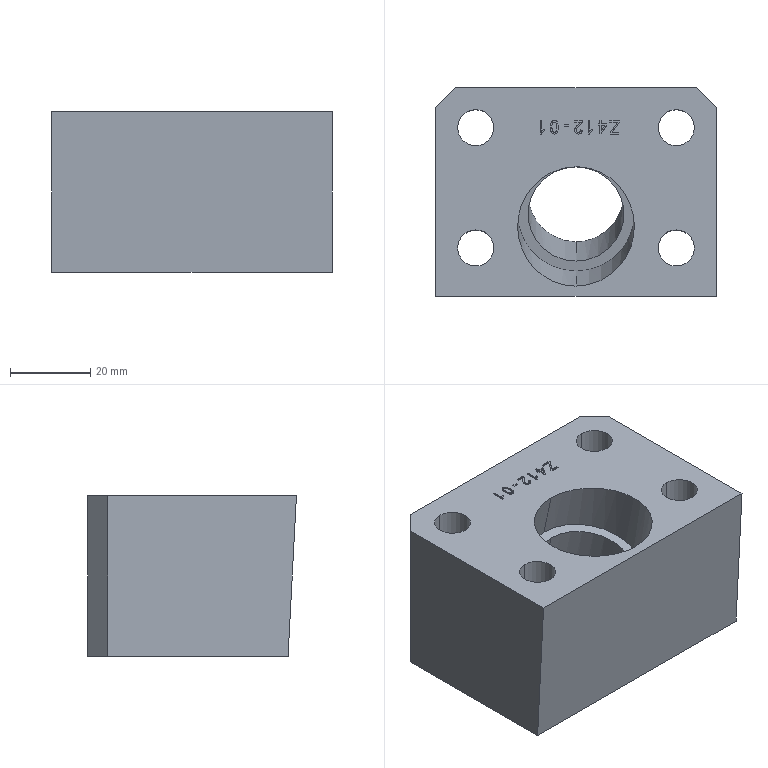Part | Creo | 1 solid | 132 faces | box 70 x 52.096 x 40 mm | volume 106812 mm3 | plane 59 | other 51 | cylinder 22 | commonest cylinder face diameters 9 x8 14 x8 24 x2 29.1 x2 2.89 x1 45.582 x1